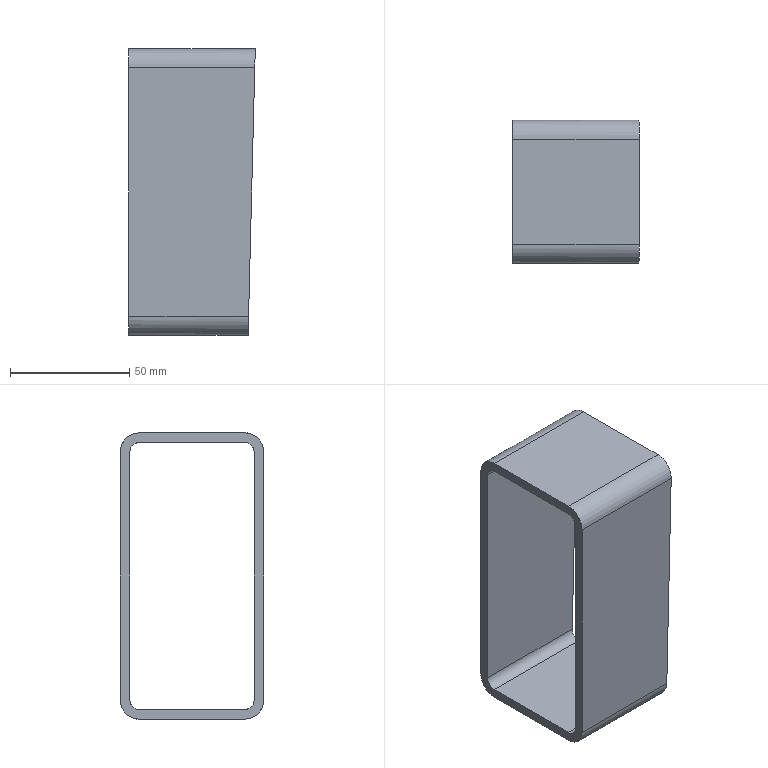Part | SolidWorks | features ICE 1, WeldMemberFeat 1, WeldmentFeature 1 | 1 solid | 18 faces | box 53 x 60 x 120 mm | volume 68742 mm3 | plane 10 | cylinder 8 | commonest cylinder face diameters 8 x4 16 x4
STEP:
#1=CARTESIAN_POINT('',(53.,22.,60.));
#2=VERTEX_POINT('',#1);
#3=CARTESIAN_POINT('',(0.,22.,60.));
#4=VERTEX_POINT('',#3);
#5=CARTESIAN_POINT('',(53.,22.,60.));
#6=DIRECTION('',(-1.,0.,0.));
#7=VECTOR('',#6,1000.);
#8=LINE('',#5,#7);
#9=EDGE_CURVE('',#2,#4,#8,.T.);
#10=ORIENTED_EDGE('',*,*,#9,.F.);
#11=CARTESIAN_POINT('',(52.8,30.,52.));
#12=VERTEX_POINT('',#11);
#13=CARTESIAN_POINT('',(53.,22.,60.));
#14=CARTESIAN_POINT('',(53.,26.686,60.));
#15=CARTESIAN_POINT('',(52.917,30.,56.686));
#16=CARTESIAN_POINT('',(52.8,30.,52.));
#17=(BOUNDED_CURVE()B_SPLINE_CURVE(3,(#13,#14,#15,#16),.UNSPECIFIED.,.F.,.F.)B_SPLINE_CURVE_WITH_KNOTS((4,4),(3.142,4.712),.UNSPECIFIED.)CURVE()GEOMETRIC_REPRESENTATION_ITEM()RATIONAL_B_SPLINE_CURVE((1.,0.8047,0.8047,1.))REPRESENTATION_ITEM(''));
#18=EDGE_CURVE('',#2,#12,#17,.T.);
#19=ORIENTED_EDGE('',*,*,#18,.T.);
#20=CARTESIAN_POINT('',(0.,30.,52.));
#21=VERTEX_POINT('',#20);
#22=CARTESIAN_POINT('',(53.,30.,52.));
#23=DIRECTION('',(-1.,0.,0.));
#24=VECTOR('',#23,1000.);
#25=LINE('',#22,#24);
#26=EDGE_CURVE('',#12,#21,#25,.T.);
#27=ORIENTED_EDGE('',*,*,#26,.T.);
#28=CARTESIAN_POINT('',(0.,22.,52.));
#29=DIRECTION('',(1.,0.,0.));
#30=DIRECTION('',(0.,0.,-1.));
#31=AXIS2_PLACEMENT_3D('',#28,#29,#30);
#32=CIRCLE('',#31,8.);
#33=EDGE_CURVE('',#21,#4,#32,.T.);
#34=ORIENTED_EDGE('',*,*,#33,.T.);
#35=EDGE_LOOP('',(#10,#19,#27,#34));
#36=FACE_OUTER_BOUND('',#35,.T.);
#37=CARTESIAN_POINT('',(53.,22.,52.));
#38=DIRECTION('',(-1.,0.,0.));
#39=DIRECTION('',(0.,0.,1.));
#40=AXIS2_PLACEMENT_3D('',#37,#38,#39);
#41=CYLINDRICAL_SURFACE('',#40,8.);
#42=ADVANCED_FACE('',(#36),#41,.T.);
#43=CARTESIAN_POINT('',(0.,-22.,60.));
#44=VERTEX_POINT('',#43);
#45=CARTESIAN_POINT('',(0.,22.,60.));
#46=DIRECTION('',(0.,-1.,0.));
#47=VECTOR('',#46,1000.);
#48=LINE('',#45,#47);
#49=EDGE_CURVE('',#4,#44,#48,.T.);
#50=ORIENTED_EDGE('',*,*,#49,.T.);
#51=CARTESIAN_POINT('',(53.,-22.,60.));
#52=VERTEX_POINT('',#51);
#53=CARTESIAN_POINT('',(53.,-22.,60.));
#54=DIRECTION('',(-1.,0.,0.));
#55=VECTOR('',#54,1000.);
#56=LINE('',#53,#55);
#57=EDGE_CURVE('',#52,#44,#56,.T.);
#58=ORIENTED_EDGE('',*,*,#57,.F.);
#59=CARTESIAN_POINT('',(53.,22.,60.));
#60=DIRECTION('',(0.,-1.,0.));
#61=VECTOR('',#60,1000.);
#62=LINE('',#59,#61);
#63=EDGE_CURVE('',#2,#52,#62,.T.);
#64=ORIENTED_EDGE('',*,*,#63,.F.);
#65=ORIENTED_EDGE('',*,*,#9,.T.);
#66=EDGE_LOOP('',(#50,#58,#64,#65));
#67=FACE_OUTER_BOUND('',#66,.T.);
#68=CARTESIAN_POINT('',(53.,22.,60.));
#69=DIRECTION('',(0.,0.,-1.));
#70=DIRECTION('',(-1.,0.,0.));
#71=AXIS2_PLACEMENT_3D('',#68,#69,#70);
#72=PLANE('',#71);
#73=ADVANCED_FACE('',(#67),#72,.F.);
#74=CARTESIAN_POINT('',(52.8,-30.,52.));
#75=VERTEX_POINT('',#74);
#76=CARTESIAN_POINT('',(0.,-30.,52.));
#77=VERTEX_POINT('',#76);
#78=CARTESIAN_POINT('',(53.,-30.,52.));
#79=DIRECTION('',(-1.,0.,0.));
#80=VECTOR('',#79,1000.);
#81=LINE('',#78,#80);
#82=EDGE_CURVE('',#75,#77,#81,.T.);
#83=ORIENTED_EDGE('',*,*,#82,.F.);
#84=CARTESIAN_POINT('',(52.8,-30.,52.));
#85=CARTESIAN_POINT('',(52.917,-30.,56.686));
#86=CARTESIAN_POINT('',(53.,-26.686,60.));
#87=CARTESIAN_POINT('',(53.,-22.,60.));
#88=(BOUNDED_CURVE()B_SPLINE_CURVE(3,(#84,#85,#86,#87),.UNSPECIFIED.,.F.,.F.)B_SPLINE_CURVE_WITH_KNOTS((4,4),(1.571,3.142),.UNSPECIFIED.)CURVE()GEOMETRIC_REPRESENTATION_ITEM()RATIONAL_B_SPLINE_CURVE((1.,0.8047,0.8047,1.))REPRESENTATION_ITEM(''));
#89=EDGE_CURVE('',#75,#52,#88,.T.);
#90=ORIENTED_EDGE('',*,*,#89,.T.);
#91=ORIENTED_EDGE('',*,*,#57,.T.);
#92=CARTESIAN_POINT('',(0.,-22.,52.));
#93=DIRECTION('',(1.,0.,0.));
#94=DIRECTION('',(0.,0.,-1.));
#95=AXIS2_PLACEMENT_3D('',#92,#93,#94);
#96=CIRCLE('',#95,8.);
#97=EDGE_CURVE('',#44,#77,#96,.T.);
#98=ORIENTED_EDGE('',*,*,#97,.T.);
#99=EDGE_LOOP('',(#83,#90,#91,#98));
#100=FACE_OUTER_BOUND('',#99,.T.);
#101=CARTESIAN_POINT('',(53.,-22.,52.));
#102=DIRECTION('',(-1.,0.,0.));
#103=DIRECTION('',(0.,0.,1.));
#104=AXIS2_PLACEMENT_3D('',#101,#102,#103);
#105=CYLINDRICAL_SURFACE('',#104,8.);
#106=ADVANCED_FACE('',(#100),#105,.T.);
#107=CARTESIAN_POINT('',(50.2,-30.,-52.));
#108=VERTEX_POINT('',#107);
#109=CARTESIAN_POINT('',(0.,-30.,-52.));
#110=VERTEX_POINT('',#109);
#111=CARTESIAN_POINT('',(53.,-30.,-52.));
#112=DIRECTION('',(-1.,0.,0.));
#113=VECTOR('',#112,1000.);
#114=LINE('',#111,#113);
#115=EDGE_CURVE('',#108,#110,#114,.T.);
#116=ORIENTED_EDGE('',*,*,#115,.F.);
#117=CARTESIAN_POINT('',(50.202,-30.,-51.93));
#118=DIRECTION('',(0.02499,0.,0.9997));
#119=VECTOR('',#118,1000.);
#120=LINE('',#117,#119);
#121=EDGE_CURVE('',#108,#75,#120,.T.);
#122=ORIENTED_EDGE('',*,*,#121,.T.);
#123=ORIENTED_EDGE('',*,*,#82,.T.);
#124=CARTESIAN_POINT('',(0.,-30.,-52.));
#125=DIRECTION('',(0.,0.,-1.));
#126=VECTOR('',#125,1000.);
#127=LINE('',#124,#126);
#128=EDGE_CURVE('',#77,#110,#127,.T.);
#129=ORIENTED_EDGE('',*,*,#128,.T.);
#130=EDGE_LOOP('',(#116,#122,#123,#129));
#131=FACE_OUTER_BOUND('',#130,.T.);
#132=CARTESIAN_POINT('',(53.,-30.,-52.));
#133=DIRECTION('',(0.,1.,0.));
#134=DIRECTION('',(0.,0.,1.));
#135=AXIS2_PLACEMENT_3D('',#132,#133,#134);
#136=PLANE('',#135);
#137=ADVANCED_FACE('',(#131),#136,.F.);
#138=CARTESIAN_POINT('',(50.,-22.,-60.));
#139=VERTEX_POINT('',#138);
#140=CARTESIAN_POINT('',(0.,-22.,-60.));
#141=VERTEX_POINT('',#140);
#142=CARTESIAN_POINT('',(53.,-22.,-60.));
#143=DIRECTION('',(-1.,0.,0.));
#144=VECTOR('',#143,1000.);
#145=LINE('',#142,#144);
#146=EDGE_CURVE('',#139,#141,#145,.T.);
#147=ORIENTED_EDGE('',*,*,#146,.F.);
#148=CARTESIAN_POINT('',(50.,-22.,-60.));
#149=CARTESIAN_POINT('',(50.,-26.686,-60.));
#150=CARTESIAN_POINT('',(50.083,-30.,-56.686));
#151=CARTESIAN_POINT('',(50.2,-30.,-52.));
#152=(BOUNDED_CURVE()B_SPLINE_CURVE(3,(#148,#149,#150,#151),.UNSPECIFIED.,.F.,.F.)B_SPLINE_CURVE_WITH_KNOTS((4,4),(0.,1.571),.UNSPECIFIED.)CURVE()GEOMETRIC_REPRESENTATION_ITEM()RATIONAL_B_SPLINE_CURVE((1.,0.8047,0.8047,1.))REPRESENTATION_ITEM(''));
#153=EDGE_CURVE('',#139,#108,#152,.T.);
#154=ORIENTED_EDGE('',*,*,#153,.T.);
#155=ORIENTED_EDGE('',*,*,#115,.T.);
#156=CARTESIAN_POINT('',(0.,-22.,-52.));
#157=DIRECTION('',(1.,0.,0.));
#158=DIRECTION('',(0.,0.,-1.));
#159=AXIS2_PLACEMENT_3D('',#156,#157,#158);
#160=CIRCLE('',#159,8.);
#161=EDGE_CURVE('',#110,#141,#160,.T.);
#162=ORIENTED_EDGE('',*,*,#161,.T.);
#163=EDGE_LOOP('',(#147,#154,#155,#162));
#164=FACE_OUTER_BOUND('',#163,.T.);
#165=CARTESIAN_POINT('',(53.,-22.,-52.));
#166=DIRECTION('',(-1.,0.,0.));
#167=DIRECTION('',(0.,0.,1.));
#168=AXIS2_PLACEMENT_3D('',#165,#166,#167);
#169=CYLINDRICAL_SURFACE('',#168,8.);
#170=ADVANCED_FACE('',(#164),#169,.T.);
#171=CARTESIAN_POINT('',(50.,22.,-60.));
#172=VERTEX_POINT('',#171);
#173=CARTESIAN_POINT('',(0.,22.,-60.));
#174=VERTEX_POINT('',#173);
#175=CARTESIAN_POINT('',(53.,22.,-60.));
#176=DIRECTION('',(-1.,0.,0.));
#177=VECTOR('',#176,1000.);
#178=LINE('',#175,#177);
#179=EDGE_CURVE('',#172,#174,#178,.T.);
#180=ORIENTED_EDGE('',*,*,#179,.F.);
#181=CARTESIAN_POINT('',(50.,30.,-60.));
#182=DIRECTION('',(0.,-1.,0.));
#183=VECTOR('',#182,1000.);
#184=LINE('',#181,#183);
#185=EDGE_CURVE('',#172,#139,#184,.T.);
#186=ORIENTED_EDGE('',*,*,#185,.T.);
#187=ORIENTED_EDGE('',*,*,#146,.T.);
#188=CARTESIAN_POINT('',(0.,-22.,-60.));
#189=DIRECTION('',(0.,1.,0.));
#190=VECTOR('',#189,1000.);
#191=LINE('',#188,#190);
#192=EDGE_CURVE('',#141,#174,#191,.T.);
#193=ORIENTED_EDGE('',*,*,#192,.T.);
#194=EDGE_LOOP('',(#180,#186,#187,#193));
#195=FACE_OUTER_BOUND('',#194,.T.);
#196=CARTESIAN_POINT('',(53.,-22.,-60.));
#197=DIRECTION('',(0.,0.,1.));
#198=DIRECTION('',(1.,0.,0.));
#199=AXIS2_PLACEMENT_3D('',#196,#197,#198);
#200=PLANE('',#199);
#201=ADVANCED_FACE('',(#195),#200,.F.);
#202=CARTESIAN_POINT('',(50.2,30.,-52.));
#203=VERTEX_POINT('',#202);
#204=CARTESIAN_POINT('',(0.,30.,-52.));
#205=VERTEX_POINT('',#204);
#206=CARTESIAN_POINT('',(53.,30.,-52.));
#207=DIRECTION('',(-1.,0.,0.));
#208=VECTOR('',#207,1000.);
#209=LINE('',#206,#208);
#210=EDGE_CURVE('',#203,#205,#209,.T.);
#211=ORIENTED_EDGE('',*,*,#210,.F.);
#212=CARTESIAN_POINT('',(50.2,30.,-52.));
#213=CARTESIAN_POINT('',(50.083,30.,-56.686));
#214=CARTESIAN_POINT('',(50.,26.686,-60.));
#215=CARTESIAN_POINT('',(50.,22.,-60.));
#216=(BOUNDED_CURVE()B_SPLINE_CURVE(3,(#212,#213,#214,#215),.UNSPECIFIED.,.F.,.F.)B_SPLINE_CURVE_WITH_KNOTS((4,4),(4.712,6.283),.UNSPECIFIED.)CURVE()GEOMETRIC_REPRESENTATION_ITEM()RATIONAL_B_SPLINE_CURVE((1.,0.8047,0.8047,1.))REPRESENTATION_ITEM(''));
#217=EDGE_CURVE('',#203,#172,#216,.T.);
#218=ORIENTED_EDGE('',*,*,#217,.T.);
#219=ORIENTED_EDGE('',*,*,#179,.T.);
#220=CARTESIAN_POINT('',(0.,22.,-52.));
#221=DIRECTION('',(1.,0.,0.));
#222=DIRECTION('',(0.,0.,-1.));
#223=AXIS2_PLACEMENT_3D('',#220,#221,#222);
#224=CIRCLE('',#223,8.);
#225=EDGE_CURVE('',#174,#205,#224,.T.);
#226=ORIENTED_EDGE('',*,*,#225,.T.);
#227=EDGE_LOOP('',(#211,#218,#219,#226));
#228=FACE_OUTER_BOUND('',#227,.T.);
#229=CARTESIAN_POINT('',(53.,22.,-52.));
#230=DIRECTION('',(-1.,0.,0.));
#231=DIRECTION('',(0.,0.,1.));
#232=AXIS2_PLACEMENT_3D('',#229,#230,#231);
#233=CYLINDRICAL_SURFACE('',#232,8.);
#234=ADVANCED_FACE('',(#228),#233,.T.);
#235=CARTESIAN_POINT('',(52.8,-26.,52.));
#236=VERTEX_POINT('',#235);
#237=CARTESIAN_POINT('',(52.9,-22.,56.));
#238=VERTEX_POINT('',#237);
#239=CARTESIAN_POINT('',(52.8,-26.,52.));
#240=CARTESIAN_POINT('',(52.859,-26.,54.343));
#241=CARTESIAN_POINT('',(52.9,-24.343,56.));
#242=CARTESIAN_POINT('',(52.9,-22.,56.));
#243=(BOUNDED_CURVE()B_SPLINE_CURVE(3,(#239,#240,#241,#242),.UNSPECIFIED.,.F.,.T.)B_SPLINE_CURVE_WITH_KNOTS((4,4),(1.571,3.142),.UNSPECIFIED.)CURVE()GEOMETRIC_REPRESENTATION_ITEM()RATIONAL_B_SPLINE_CURVE((1.,0.8047,0.8047,1.))REPRESENTATION_ITEM(''));
#244=EDGE_CURVE('',#236,#238,#243,.T.);
#245=ORIENTED_EDGE('',*,*,#244,.F.);
#246=CARTESIAN_POINT('',(0.,-26.,52.));
#247=VERTEX_POINT('',#246);
#248=CARTESIAN_POINT('',(53.,-26.,52.));
#249=DIRECTION('',(-1.,0.,0.));
#250=VECTOR('',#249,1000.);
#251=LINE('',#248,#250);
#252=EDGE_CURVE('',#236,#247,#251,.T.);
#253=ORIENTED_EDGE('',*,*,#252,.T.);
#254=CARTESIAN_POINT('',(0.,-22.,56.));
#255=VERTEX_POINT('',#254);
#256=CARTESIAN_POINT('',(0.,-22.,52.));
#257=DIRECTION('',(1.,0.,0.));
#258=DIRECTION('',(0.,0.,-1.));
#259=AXIS2_PLACEMENT_3D('',#256,#257,#258);
#260=CIRCLE('',#259,4.);
#261=EDGE_CURVE('',#255,#247,#260,.T.);
#262=ORIENTED_EDGE('',*,*,#261,.F.);
#263=CARTESIAN_POINT('',(53.,-22.,56.));
#264=DIRECTION('',(-1.,0.,0.));
#265=VECTOR('',#264,1000.);
#266=LINE('',#263,#265);
#267=EDGE_CURVE('',#238,#255,#266,.T.);
#268=ORIENTED_EDGE('',*,*,#267,.F.);
#269=EDGE_LOOP('',(#245,#253,#262,#268));
#270=FACE_OUTER_BOUND('',#269,.T.);
#271=CARTESIAN_POINT('',(53.,-22.,52.));
#272=DIRECTION('',(-1.,0.,0.));
#273=DIRECTION('',(0.,0.,1.));
#274=AXIS2_PLACEMENT_3D('',#271,#272,#273);
#275=CYLINDRICAL_SURFACE('',#274,4.);
#276=ADVANCED_FACE('',(#270),#275,.F.);
#277=CARTESIAN_POINT('',(52.9,22.,56.));
#278=VERTEX_POINT('',#277);
#279=CARTESIAN_POINT('',(52.9,22.,56.));
#280=DIRECTION('',(0.,1.,0.));
#281=VECTOR('',#280,1000.);
#282=LINE('',#279,#281);
#283=EDGE_CURVE('',#238,#278,#282,.T.);
#284=ORIENTED_EDGE('',*,*,#283,.F.);
#285=ORIENTED_EDGE('',*,*,#267,.T.);
#286=CARTESIAN_POINT('',(0.,22.,56.));
#287=VERTEX_POINT('',#286);
#288=CARTESIAN_POINT('',(0.,22.,56.));
#289=DIRECTION('',(0.,-1.,0.));
#290=VECTOR('',#289,1000.);
#291=LINE('',#288,#290);
#292=EDGE_CURVE('',#287,#255,#291,.T.);
#293=ORIENTED_EDGE('',*,*,#292,.F.);
#294=CARTESIAN_POINT('',(53.,22.,56.));
#295=DIRECTION('',(-1.,0.,0.));
#296=VECTOR('',#295,1000.);
#297=LINE('',#294,#296);
#298=EDGE_CURVE('',#278,#287,#297,.T.);
#299=ORIENTED_EDGE('',*,*,#298,.F.);
#300=EDGE_LOOP('',(#284,#285,#293,#299));
#301=FACE_OUTER_BOUND('',#300,.T.);
#302=CARTESIAN_POINT('',(53.,22.,56.));
#303=DIRECTION('',(0.,0.,-1.));
#304=DIRECTION('',(-1.,0.,0.));
#305=AXIS2_PLACEMENT_3D('',#302,#303,#304);
#306=PLANE('',#305);
#307=ADVANCED_FACE('',(#301),#306,.T.);
#308=CARTESIAN_POINT('',(52.8,26.,52.));
#309=VERTEX_POINT('',#308);
#310=CARTESIAN_POINT('',(52.9,22.,56.));
#311=CARTESIAN_POINT('',(52.9,24.343,56.));
#312=CARTESIAN_POINT('',(52.859,26.,54.343));
#313=CARTESIAN_POINT('',(52.8,26.,52.));
#314=(BOUNDED_CURVE()B_SPLINE_CURVE(3,(#310,#311,#312,#313),.UNSPECIFIED.,.F.,.F.)B_SPLINE_CURVE_WITH_KNOTS((4,4),(3.142,4.712),.UNSPECIFIED.)CURVE()GEOMETRIC_REPRESENTATION_ITEM()RATIONAL_B_SPLINE_CURVE((1.,0.8047,0.8047,1.))REPRESENTATION_ITEM(''));
#315=EDGE_CURVE('',#278,#309,#314,.T.);
#316=ORIENTED_EDGE('',*,*,#315,.F.);
#317=ORIENTED_EDGE('',*,*,#298,.T.);
#318=CARTESIAN_POINT('',(0.,26.,52.));
#319=VERTEX_POINT('',#318);
#320=CARTESIAN_POINT('',(0.,22.,52.));
#321=DIRECTION('',(1.,0.,0.));
#322=DIRECTION('',(0.,0.,-1.));
#323=AXIS2_PLACEMENT_3D('',#320,#321,#322);
#324=CIRCLE('',#323,4.);
#325=EDGE_CURVE('',#319,#287,#324,.T.);
#326=ORIENTED_EDGE('',*,*,#325,.F.);
#327=CARTESIAN_POINT('',(53.,26.,52.));
#328=DIRECTION('',(-1.,0.,0.));
#329=VECTOR('',#328,1000.);
#330=LINE('',#327,#329);
#331=EDGE_CURVE('',#309,#319,#330,.T.);
#332=ORIENTED_EDGE('',*,*,#331,.F.);
#333=EDGE_LOOP('',(#316,#317,#326,#332));
#334=FACE_OUTER_BOUND('',#333,.T.);
#335=CARTESIAN_POINT('',(53.,22.,52.));
#336=DIRECTION('',(-1.,0.,0.));
#337=DIRECTION('',(0.,0.,1.));
#338=AXIS2_PLACEMENT_3D('',#335,#336,#337);
#339=CYLINDRICAL_SURFACE('',#338,4.);
#340=ADVANCED_FACE('',(#334),#339,.F.);
#341=CARTESIAN_POINT('',(50.2,26.,-52.));
#342=VERTEX_POINT('',#341);
#343=CARTESIAN_POINT('',(52.8,26.,52.005));
#344=DIRECTION('',(-0.02499,0.,-0.9997));
#345=VECTOR('',#344,1000.);
#346=LINE('',#343,#345);
#347=EDGE_CURVE('',#309,#342,#346,.T.);
#348=ORIENTED_EDGE('',*,*,#347,.F.);
#349=ORIENTED_EDGE('',*,*,#331,.T.);
#350=CARTESIAN_POINT('',(0.,26.,-52.));
#351=VERTEX_POINT('',#350);
#352=CARTESIAN_POINT('',(0.,26.,52.));
#353=DIRECTION('',(0.,0.,1.));
#354=VECTOR('',#353,1000.);
#355=LINE('',#352,#354);
#356=EDGE_CURVE('',#351,#319,#355,.T.);
#357=ORIENTED_EDGE('',*,*,#356,.F.);
#358=CARTESIAN_POINT('',(53.,26.,-52.));
#359=DIRECTION('',(-1.,0.,0.));
#360=VECTOR('',#359,1000.);
#361=LINE('',#358,#360);
#362=EDGE_CURVE('',#342,#351,#361,.T.);
#363=ORIENTED_EDGE('',*,*,#362,.F.);
#364=EDGE_LOOP('',(#348,#349,#357,#363));
#365=FACE_OUTER_BOUND('',#364,.T.);
#366=CARTESIAN_POINT('',(53.,26.,52.));
#367=DIRECTION('',(0.,-1.,0.));
#368=DIRECTION('',(0.,0.,-1.));
#369=AXIS2_PLACEMENT_3D('',#366,#367,#368);
#370=PLANE('',#369);
#371=ADVANCED_FACE('',(#365),#370,.T.);
#372=CARTESIAN_POINT('',(50.1,22.,-56.));
#373=VERTEX_POINT('',#372);
#374=CARTESIAN_POINT('',(50.2,26.,-52.));
#375=CARTESIAN_POINT('',(50.141,26.,-54.343));
#376=CARTESIAN_POINT('',(50.1,24.343,-56.));
#377=CARTESIAN_POINT('',(50.1,22.,-56.));
#378=(BOUNDED_CURVE()B_SPLINE_CURVE(3,(#374,#375,#376,#377),.UNSPECIFIED.,.F.,.F.)B_SPLINE_CURVE_WITH_KNOTS((4,4),(4.712,6.283),.UNSPECIFIED.)CURVE()GEOMETRIC_REPRESENTATION_ITEM()RATIONAL_B_SPLINE_CURVE((1.,0.8047,0.8047,1.))REPRESENTATION_ITEM(''));
#379=EDGE_CURVE('',#342,#373,#378,.T.);
#380=ORIENTED_EDGE('',*,*,#379,.F.);
#381=ORIENTED_EDGE('',*,*,#362,.T.);
#382=CARTESIAN_POINT('',(0.,22.,-56.));
#383=VERTEX_POINT('',#382);
#384=CARTESIAN_POINT('',(0.,22.,-52.));
#385=DIRECTION('',(1.,0.,0.));
#386=DIRECTION('',(0.,0.,-1.));
#387=AXIS2_PLACEMENT_3D('',#384,#385,#386);
#388=CIRCLE('',#387,4.);
#389=EDGE_CURVE('',#383,#351,#388,.T.);
#390=ORIENTED_EDGE('',*,*,#389,.F.);
#391=CARTESIAN_POINT('',(53.,22.,-56.));
#392=DIRECTION('',(-1.,0.,0.));
#393=VECTOR('',#392,1000.);
#394=LINE('',#391,#393);
#395=EDGE_CURVE('',#373,#383,#394,.T.);
#396=ORIENTED_EDGE('',*,*,#395,.F.);
#397=EDGE_LOOP('',(#380,#381,#390,#396));
#398=FACE_OUTER_BOUND('',#397,.T.);
#399=CARTESIAN_POINT('',(53.,22.,-52.));
#400=DIRECTION('',(-1.,0.,0.));
#401=DIRECTION('',(0.,0.,1.));
#402=AXIS2_PLACEMENT_3D('',#399,#400,#401);
#403=CYLINDRICAL_SURFACE('',#402,4.);
#404=ADVANCED_FACE('',(#398),#403,.F.);
#405=CARTESIAN_POINT('',(50.1,-22.,-56.));
#406=VERTEX_POINT('',#405);
#407=CARTESIAN_POINT('',(50.1,-22.,-56.));
#408=DIRECTION('',(0.,-1.,0.));
#409=VECTOR('',#408,1000.);
#410=LINE('',#407,#409);
#411=EDGE_CURVE('',#373,#406,#410,.T.);
#412=ORIENTED_EDGE('',*,*,#411,.F.);
#413=ORIENTED_EDGE('',*,*,#395,.T.);
#414=CARTESIAN_POINT('',(0.,-22.,-56.));
#415=VERTEX_POINT('',#414);
#416=CARTESIAN_POINT('',(0.,-22.,-56.));
#417=DIRECTION('',(0.,1.,0.));
#418=VECTOR('',#417,1000.);
#419=LINE('',#416,#418);
#420=EDGE_CURVE('',#415,#383,#419,.T.);
#421=ORIENTED_EDGE('',*,*,#420,.F.);
#422=CARTESIAN_POINT('',(53.,-22.,-56.));
#423=DIRECTION('',(-1.,0.,0.));
#424=VECTOR('',#423,1000.);
#425=LINE('',#422,#424);
#426=EDGE_CURVE('',#406,#415,#425,.T.);
#427=ORIENTED_EDGE('',*,*,#426,.F.);
#428=EDGE_LOOP('',(#412,#413,#421,#427));
#429=FACE_OUTER_BOUND('',#428,.T.);
#430=CARTESIAN_POINT('',(53.,-22.,-56.));
#431=DIRECTION('',(0.,0.,1.));
#432=DIRECTION('',(1.,0.,0.));
#433=AXIS2_PLACEMENT_3D('',#430,#431,#432);
#434=PLANE('',#433);
#435=ADVANCED_FACE('',(#429),#434,.T.);
#436=CARTESIAN_POINT('',(50.2,-26.,-52.));
#437=VERTEX_POINT('',#436);
#438=CARTESIAN_POINT('',(50.1,-22.,-56.));
#439=CARTESIAN_POINT('',(50.1,-24.343,-56.));
#440=CARTESIAN_POINT('',(50.141,-26.,-54.343));
#441=CARTESIAN_POINT('',(50.2,-26.,-52.));
#442=(BOUNDED_CURVE()B_SPLINE_CURVE(3,(#438,#439,#440,#441),.UNSPECIFIED.,.F.,.F.)B_SPLINE_CURVE_WITH_KNOTS((4,4),(0.,1.571),.UNSPECIFIED.)CURVE()GEOMETRIC_REPRESENTATION_ITEM()RATIONAL_B_SPLINE_CURVE((1.,0.8047,0.8047,1.))REPRESENTATION_ITEM(''));
#443=EDGE_CURVE('',#406,#437,#442,.T.);
#444=ORIENTED_EDGE('',*,*,#443,.F.);
#445=ORIENTED_EDGE('',*,*,#426,.T.);
#446=CARTESIAN_POINT('',(0.,-26.,-52.));
#447=VERTEX_POINT('',#446);
#448=CARTESIAN_POINT('',(0.,-22.,-52.));
#449=DIRECTION('',(1.,0.,0.));
#450=DIRECTION('',(0.,0.,-1.));
#451=AXIS2_PLACEMENT_3D('',#448,#449,#450);
#452=CIRCLE('',#451,4.);
#453=EDGE_CURVE('',#447,#415,#452,.T.);
#454=ORIENTED_EDGE('',*,*,#453,.F.);
#455=CARTESIAN_POINT('',(53.,-26.,-52.));
#456=DIRECTION('',(-1.,0.,0.));
#457=VECTOR('',#456,1000.);
#458=LINE('',#455,#457);
#459=EDGE_CURVE('',#437,#447,#458,.T.);
#460=ORIENTED_EDGE('',*,*,#459,.F.);
#461=EDGE_LOOP('',(#444,#445,#454,#460));
#462=FACE_OUTER_BOUND('',#461,.T.);
#463=CARTESIAN_POINT('',(53.,-22.,-52.));
#464=DIRECTION('',(-1.,0.,0.));
#465=DIRECTION('',(0.,0.,1.));
#466=AXIS2_PLACEMENT_3D('',#463,#464,#465);
#467=CYLINDRICAL_SURFACE('',#466,4.);
#468=ADVANCED_FACE('',(#462),#467,.F.);
#469=CARTESIAN_POINT('',(50.202,-26.,-51.93));
#470=DIRECTION('',(0.02499,0.,0.9997));
#471=VECTOR('',#470,1000.);
#472=LINE('',#469,#471);
#473=EDGE_CURVE('',#437,#236,#472,.T.);
#474=ORIENTED_EDGE('',*,*,#473,.F.);
#475=ORIENTED_EDGE('',*,*,#459,.T.);
#476=CARTESIAN_POINT('',(0.,-26.,-52.));
#477=DIRECTION('',(0.,0.,-1.));
#478=VECTOR('',#477,1000.);
#479=LINE('',#476,#478);
#480=EDGE_CURVE('',#247,#447,#479,.T.);
#481=ORIENTED_EDGE('',*,*,#480,.F.);
#482=ORIENTED_EDGE('',*,*,#252,.F.);
#483=EDGE_LOOP('',(#474,#475,#481,#482));
#484=FACE_OUTER_BOUND('',#483,.T.);
#485=CARTESIAN_POINT('',(53.,-26.,-52.));
#486=DIRECTION('',(0.,1.,0.));
#487=DIRECTION('',(0.,0.,1.));
#488=AXIS2_PLACEMENT_3D('',#485,#486,#487);
#489=PLANE('',#488);
#490=ADVANCED_FACE('',(#484),#489,.T.);
#491=ORIENTED_EDGE('',*,*,#26,.F.);
#492=CARTESIAN_POINT('',(53.,30.,60.));
#493=DIRECTION('',(-0.02499,0.,-0.9997));
#494=VECTOR('',#493,1000.);
#495=LINE('',#492,#494);
#496=EDGE_CURVE('',#12,#203,#495,.T.);
#497=ORIENTED_EDGE('',*,*,#496,.T.);
#498=ORIENTED_EDGE('',*,*,#210,.T.);
#499=CARTESIAN_POINT('',(0.,30.,52.));
#500=DIRECTION('',(0.,0.,1.));
#501=VECTOR('',#500,1000.);
#502=LINE('',#499,#501);
#503=EDGE_CURVE('',#205,#21,#502,.T.);
#504=ORIENTED_EDGE('',*,*,#503,.T.);
#505=EDGE_LOOP('',(#491,#497,#498,#504));
#506=FACE_OUTER_BOUND('',#505,.T.);
#507=CARTESIAN_POINT('',(53.,30.,52.));
#508=DIRECTION('',(0.,-1.,0.));
#509=DIRECTION('',(0.,0.,-1.));
#510=AXIS2_PLACEMENT_3D('',#507,#508,#509);
#511=PLANE('',#510);
#512=ADVANCED_FACE('',(#506),#511,.F.);
#513=ORIENTED_EDGE('',*,*,#261,.T.);
#514=ORIENTED_EDGE('',*,*,#480,.T.);
#515=ORIENTED_EDGE('',*,*,#453,.T.);
#516=ORIENTED_EDGE('',*,*,#420,.T.);
#517=ORIENTED_EDGE('',*,*,#389,.T.);
#518=ORIENTED_EDGE('',*,*,#356,.T.);
#519=ORIENTED_EDGE('',*,*,#325,.T.);
#520=ORIENTED_EDGE('',*,*,#292,.T.);
#521=EDGE_LOOP('',(#513,#514,#515,#516,#517,#518,#519,#520));
#522=FACE_BOUND('',#521,.T.);
#523=ORIENTED_EDGE('',*,*,#33,.F.);
#524=ORIENTED_EDGE('',*,*,#503,.F.);
#525=ORIENTED_EDGE('',*,*,#225,.F.);
#526=ORIENTED_EDGE('',*,*,#192,.F.);
#527=ORIENTED_EDGE('',*,*,#161,.F.);
#528=ORIENTED_EDGE('',*,*,#128,.F.);
#529=ORIENTED_EDGE('',*,*,#97,.F.);
#530=ORIENTED_EDGE('',*,*,#49,.F.);
#531=EDGE_LOOP('',(#523,#524,#525,#526,#527,#528,#529,#530));
#532=FACE_OUTER_BOUND('',#531,.T.);
#533=CARTESIAN_POINT('',(0.,22.,52.));
#534=DIRECTION('',(1.,0.,0.));
#535=DIRECTION('',(0.,0.,-1.));
#536=AXIS2_PLACEMENT_3D('',#533,#534,#535);
#537=PLANE('',#536);
#538=ADVANCED_FACE('',(#522,#532),#537,.F.);
#539=ORIENTED_EDGE('',*,*,#244,.T.);
#540=ORIENTED_EDGE('',*,*,#283,.T.);
#541=ORIENTED_EDGE('',*,*,#315,.T.);
#542=ORIENTED_EDGE('',*,*,#347,.T.);
#543=ORIENTED_EDGE('',*,*,#379,.T.);
#544=ORIENTED_EDGE('',*,*,#411,.T.);
#545=ORIENTED_EDGE('',*,*,#443,.T.);
#546=ORIENTED_EDGE('',*,*,#473,.T.);
#547=EDGE_LOOP('',(#539,#540,#541,#542,#543,#544,#545,#546));
#548=FACE_BOUND('',#547,.T.);
#549=ORIENTED_EDGE('',*,*,#63,.T.);
#550=ORIENTED_EDGE('',*,*,#89,.F.);
#551=ORIENTED_EDGE('',*,*,#121,.F.);
#552=ORIENTED_EDGE('',*,*,#153,.F.);
#553=ORIENTED_EDGE('',*,*,#185,.F.);
#554=ORIENTED_EDGE('',*,*,#217,.F.);
#555=ORIENTED_EDGE('',*,*,#496,.F.);
#556=ORIENTED_EDGE('',*,*,#18,.F.);
#557=EDGE_LOOP('',(#549,#550,#551,#552,#553,#554,#555,#556));
#558=FACE_OUTER_BOUND('',#557,.T.);
#559=CARTESIAN_POINT('',(53.,30.,60.));
#560=DIRECTION('',(-0.9997,0.,0.02499));
#561=DIRECTION('',(0.02499,0.,0.9997));
#562=AXIS2_PLACEMENT_3D('',#559,#560,#561);
#563=PLANE('',#562);
#564=ADVANCED_FACE('',(#548,#558),#563,.F.);
#565=CLOSED_SHELL('',(#42,#73,#106,#137,#170,#201,#234,#276,#307,#340,#371,#404,#435,#468,#490,#512,#538,#564));
#566=MANIFOLD_SOLID_BREP('',#565);
#567=CARTESIAN_POINT('',(0.,0.,0.));
#568=DIRECTION('',(0.,0.,1.));
#569=DIRECTION('',(1.,0.,0.));
#570=AXIS2_PLACEMENT_3D('',#567,#568,#569);
#571=(LENGTH_UNIT()NAMED_UNIT(*)SI_UNIT(.MILLI.,.METRE.));
#572=UNCERTAINTY_MEASURE_WITH_UNIT(LENGTH_MEASURE(0.00001),#571,'','');
#573=(NAMED_UNIT(*)PLANE_ANGLE_UNIT()SI_UNIT($,.RADIAN.));
#574=(NAMED_UNIT(*)SI_UNIT($,.STERADIAN.)SOLID_ANGLE_UNIT());
#575=(GEOMETRIC_REPRESENTATION_CONTEXT(3)GLOBAL_UNCERTAINTY_ASSIGNED_CONTEXT((#572))GLOBAL_UNIT_ASSIGNED_CONTEXT((#571,#573,#574))REPRESENTATION_CONTEXT('',''));
#576=ADVANCED_BREP_SHAPE_REPRESENTATION('',(#566,#570),#575);